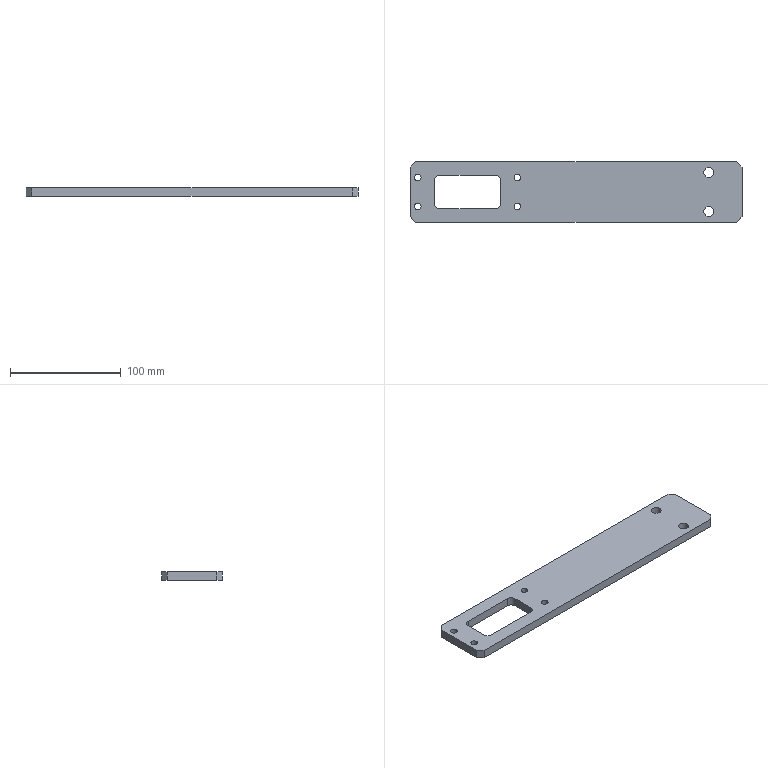Part | STEP file | Cable Carrier Bracket 2 | 1 solid | 30 faces | box 300 x 55 x 8 mm | volume 115449 mm3 | cylinder 16 | plane 14 | commonest cylinder face diameters 6 x8 9 x4 10 x4